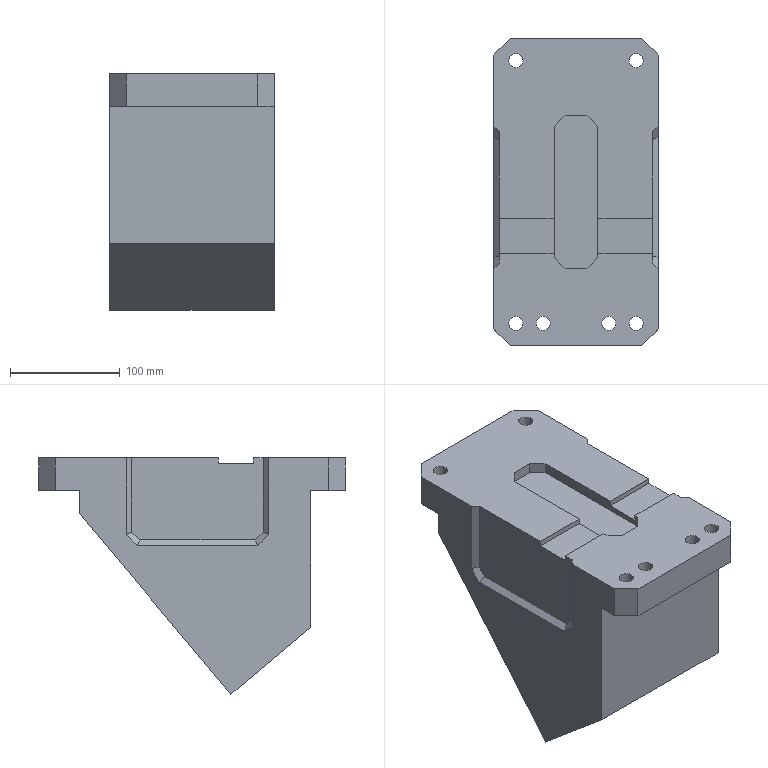Part | NX | features solid 2 | 1 solid | 57 faces | box 150 x 280 x 215.84 mm | volume 4894964 mm3 | plane 47 | cylinder 10 | commonest cylinder face diameters 13 x6 20 x4